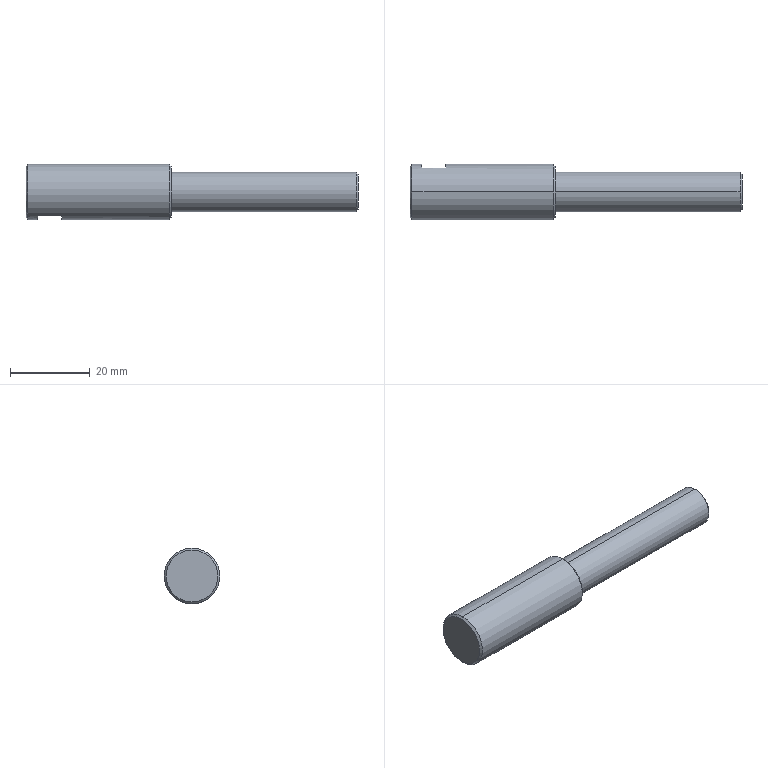Part | STEP file | 0243_216_Shaft | 1 solid | 19 faces | box 83.5 x 14 x 14 mm | volume 9237 mm3 | plane 9 | cone 6 | cylinder 4 | commonest cylinder face diameters 10 x2 14 x2
STEP:
#1=CARTESIAN_POINT('',(0.,0.,0.));
#2=DIRECTION('',(0.,0.,1.));
#3=DIRECTION('',(1.,0.,0.));
#4=AXIS2_PLACEMENT_3D('',#1,#2,#3);
#5=CARTESIAN_POINT('',(47.,0.,-4.5));
#6=VERTEX_POINT('',#5);
#7=CARTESIAN_POINT('',(47.,0.,4.5));
#8=VERTEX_POINT('',#7);
#9=CARTESIAN_POINT('',(47.,0.,0.));
#10=DIRECTION('',(1.,0.,0.));
#11=DIRECTION('',(0.,0.,1.));
#12=AXIS2_PLACEMENT_3D('',#9,#10,#11);
#13=CIRCLE('',#12,4.5);
#14=CARTESIAN_POINT('',(46.5,0.,0.));
#15=DIRECTION('',(-1.,0.,0.));
#16=DIRECTION('',(0.,0.,1.));
#17=AXIS2_PLACEMENT_3D('',#14,#15,#16);
#18=CONICAL_SURFACE('',#17,5.,0.7854);
#19=CARTESIAN_POINT('',(6.283,-0.5));
#20=DIRECTION('',(-1.,0.));
#21=VECTOR('',#20,1.);
#22=LINE('',#19,#21);
#23=(GEOMETRIC_REPRESENTATION_CONTEXT(2)PARAMETRIC_REPRESENTATION_CONTEXT()REPRESENTATION_CONTEXT('',''));
#24=DEFINITIONAL_REPRESENTATION('',(#22),#23);
#25=PCURVE('',#18,#24);
#26=CARTESIAN_POINT('',(47.,0.,0.));
#27=DIRECTION('',(-1.,0.,0.));
#28=DIRECTION('',(0.,0.,1.));
#29=AXIS2_PLACEMENT_3D('',#26,#27,#28);
#30=PLANE('',#29);
#31=CARTESIAN_POINT('',(4.5,0.));
#32=CARTESIAN_POINT('',(4.5,-7.794));
#33=CARTESIAN_POINT('',(-2.25,-3.897));
#34=CARTESIAN_POINT('',(-9.,0.));
#35=CARTESIAN_POINT('',(-2.25,3.897));
#36=CARTESIAN_POINT('',(4.5,7.794));
#37=CARTESIAN_POINT('',(4.5,0.));
#38=(BOUNDED_CURVE()B_SPLINE_CURVE(2,(#31,#32,#33,#34,#35,#36,#37),.UNSPECIFIED.,.T.,.F.)B_SPLINE_CURVE_WITH_KNOTS((1,2,2,2,2,1),(-2.094,0.,2.094,4.189,6.283,8.378),.UNSPECIFIED.)CURVE()GEOMETRIC_REPRESENTATION_ITEM()RATIONAL_B_SPLINE_CURVE((1.,0.5,1.,0.5,1.,0.5,1.))REPRESENTATION_ITEM(''));
#39=(GEOMETRIC_REPRESENTATION_CONTEXT(2)PARAMETRIC_REPRESENTATION_CONTEXT()REPRESENTATION_CONTEXT('',''));
#40=DEFINITIONAL_REPRESENTATION('',(#38),#39);
#41=PCURVE('',#30,#40);
#42=SURFACE_CURVE('',#13,(#25,#41),.PCURVE_S1.);
#43=EDGE_CURVE('',#6,#8,#42,.T.);
#44=ORIENTED_EDGE('',*,*,#43,.F.);
#45=CARTESIAN_POINT('',(46.5,0.,-5.));
#46=VERTEX_POINT('',#45);
#47=CARTESIAN_POINT('',(46.5,0.,-5.));
#48=DIRECTION('',(-0.7071,0.,-0.7071));
#49=VECTOR('',#48,1.);
#50=LINE('',#47,#49);
#51=CARTESIAN_POINT('',(3.142,0.));
#52=DIRECTION('',(0.,1.));
#53=VECTOR('',#52,1.);
#54=LINE('',#51,#53);
#55=(GEOMETRIC_REPRESENTATION_CONTEXT(2)PARAMETRIC_REPRESENTATION_CONTEXT()REPRESENTATION_CONTEXT('',''));
#56=DEFINITIONAL_REPRESENTATION('',(#54),#55);
#57=PCURVE('',#18,#56);
#58=CARTESIAN_POINT('',(46.5,0.,0.));
#59=DIRECTION('',(-1.,0.,0.));
#60=DIRECTION('',(0.,0.,1.));
#61=AXIS2_PLACEMENT_3D('',#58,#59,#60);
#62=CONICAL_SURFACE('',#61,5.,0.7854);
#63=CARTESIAN_POINT('',(3.142,0.));
#64=DIRECTION('',(0.,1.));
#65=VECTOR('',#64,1.);
#66=LINE('',#63,#65);
#67=(GEOMETRIC_REPRESENTATION_CONTEXT(2)PARAMETRIC_REPRESENTATION_CONTEXT()REPRESENTATION_CONTEXT('',''));
#68=DEFINITIONAL_REPRESENTATION('',(#66),#67);
#69=PCURVE('',#62,#68);
#70=SURFACE_CURVE('',#50,(#57,#69),.PCURVE_S1.);
#71=EDGE_CURVE('',#6,#46,#70,.T.);
#72=ORIENTED_EDGE('',*,*,#71,.T.);
#73=CARTESIAN_POINT('',(46.5,0.,5.));
#74=VERTEX_POINT('',#73);
#75=CARTESIAN_POINT('',(46.5,0.,0.));
#76=DIRECTION('',(-1.,0.,0.));
#77=DIRECTION('',(0.,0.,1.));
#78=AXIS2_PLACEMENT_3D('',#75,#76,#77);
#79=CIRCLE('',#78,5.);
#80=CARTESIAN_POINT('',(0.,0.));
#81=DIRECTION('',(1.,0.));
#82=VECTOR('',#81,1.);
#83=LINE('',#80,#82);
#84=(GEOMETRIC_REPRESENTATION_CONTEXT(2)PARAMETRIC_REPRESENTATION_CONTEXT()REPRESENTATION_CONTEXT('',''));
#85=DEFINITIONAL_REPRESENTATION('',(#83),#84);
#86=PCURVE('',#18,#85);
#87=CARTESIAN_POINT('',(-41.827,0.,0.));
#88=DIRECTION('',(-1.,0.,0.));
#89=DIRECTION('',(0.,0.,1.));
#90=AXIS2_PLACEMENT_3D('',#87,#88,#89);
#91=CYLINDRICAL_SURFACE('',#90,5.);
#92=CARTESIAN_POINT('',(0.,-88.327));
#93=DIRECTION('',(1.,0.));
#94=VECTOR('',#93,1.);
#95=LINE('',#92,#94);
#96=(GEOMETRIC_REPRESENTATION_CONTEXT(2)PARAMETRIC_REPRESENTATION_CONTEXT()REPRESENTATION_CONTEXT('',''));
#97=DEFINITIONAL_REPRESENTATION('',(#95),#96);
#98=PCURVE('',#91,#97);
#99=SURFACE_CURVE('',#79,(#86,#98),.PCURVE_S1.);
#100=EDGE_CURVE('',#74,#46,#99,.T.);
#101=ORIENTED_EDGE('',*,*,#100,.F.);
#102=CARTESIAN_POINT('',(46.5,0.,5.));
#103=DIRECTION('',(-0.7071,0.,0.7071));
#104=VECTOR('',#103,1.);
#105=LINE('',#102,#104);
#106=CARTESIAN_POINT('',(0.,0.));
#107=DIRECTION('',(0.,1.));
#108=VECTOR('',#107,1.);
#109=LINE('',#106,#108);
#110=(GEOMETRIC_REPRESENTATION_CONTEXT(2)PARAMETRIC_REPRESENTATION_CONTEXT()REPRESENTATION_CONTEXT('',''));
#111=DEFINITIONAL_REPRESENTATION('',(#109),#110);
#112=PCURVE('',#18,#111);
#113=CARTESIAN_POINT('',(6.283,0.));
#114=DIRECTION('',(0.,1.));
#115=VECTOR('',#114,1.);
#116=LINE('',#113,#115);
#117=(GEOMETRIC_REPRESENTATION_CONTEXT(2)PARAMETRIC_REPRESENTATION_CONTEXT()REPRESENTATION_CONTEXT('',''));
#118=DEFINITIONAL_REPRESENTATION('',(#116),#117);
#119=PCURVE('',#62,#118);
#120=SURFACE_CURVE('',#105,(#112,#119),.PCURVE_S1.);
#121=EDGE_CURVE('',#8,#74,#120,.T.);
#122=ORIENTED_EDGE('',*,*,#121,.F.);
#123=EDGE_LOOP('',(#44,#72,#101,#122));
#124=FACE_BOUND('',#123,.T.);
#125=ADVANCED_FACE('',(#124),#18,.T.);
#126=CARTESIAN_POINT('',(0.,0.,-6.5));
#127=VERTEX_POINT('',#126);
#128=CARTESIAN_POINT('',(0.,0.,6.5));
#129=VERTEX_POINT('',#128);
#130=CARTESIAN_POINT('',(0.,0.,0.));
#131=DIRECTION('',(1.,0.,0.));
#132=DIRECTION('',(0.,0.,1.));
#133=AXIS2_PLACEMENT_3D('',#130,#131,#132);
#134=CIRCLE('',#133,6.5);
#135=CARTESIAN_POINT('',(-0.5,0.,0.));
#136=DIRECTION('',(-1.,0.,0.));
#137=DIRECTION('',(0.,0.,1.));
#138=AXIS2_PLACEMENT_3D('',#135,#136,#137);
#139=CONICAL_SURFACE('',#138,7.,0.7854);
#140=CARTESIAN_POINT('',(6.283,-0.5));
#141=DIRECTION('',(-1.,0.));
#142=VECTOR('',#141,1.);
#143=LINE('',#140,#142);
#144=(GEOMETRIC_REPRESENTATION_CONTEXT(2)PARAMETRIC_REPRESENTATION_CONTEXT()REPRESENTATION_CONTEXT('',''));
#145=DEFINITIONAL_REPRESENTATION('',(#143),#144);
#146=PCURVE('',#139,#145);
#147=CARTESIAN_POINT('',(0.,5.,0.));
#148=DIRECTION('',(-1.,0.,0.));
#149=DIRECTION('',(0.,0.,1.));
#150=AXIS2_PLACEMENT_3D('',#147,#148,#149);
#151=PLANE('',#150);
#152=CARTESIAN_POINT('',(6.5,-5.));
#153=CARTESIAN_POINT('',(6.5,-16.258));
#154=CARTESIAN_POINT('',(-3.25,-10.629));
#155=CARTESIAN_POINT('',(-13.,-5.));
#156=CARTESIAN_POINT('',(-3.25,0.6292));
#157=CARTESIAN_POINT('',(6.5,6.258));
#158=CARTESIAN_POINT('',(6.5,-5.));
#159=(BOUNDED_CURVE()B_SPLINE_CURVE(2,(#152,#153,#154,#155,#156,#157,#158),.UNSPECIFIED.,.T.,.F.)B_SPLINE_CURVE_WITH_KNOTS((1,2,2,2,2,1),(-2.094,0.,2.094,4.189,6.283,8.378),.UNSPECIFIED.)CURVE()GEOMETRIC_REPRESENTATION_ITEM()RATIONAL_B_SPLINE_CURVE((1.,0.5,1.,0.5,1.,0.5,1.))REPRESENTATION_ITEM(''));
#160=(GEOMETRIC_REPRESENTATION_CONTEXT(2)PARAMETRIC_REPRESENTATION_CONTEXT()REPRESENTATION_CONTEXT('',''));
#161=DEFINITIONAL_REPRESENTATION('',(#159),#160);
#162=PCURVE('',#151,#161);
#163=SURFACE_CURVE('',#134,(#146,#162),.PCURVE_S1.);
#164=EDGE_CURVE('',#127,#129,#163,.T.);
#165=ORIENTED_EDGE('',*,*,#164,.F.);
#166=CARTESIAN_POINT('',(-0.5,0.,-7.));
#167=VERTEX_POINT('',#166);
#168=CARTESIAN_POINT('',(-0.5,0.,-7.));
#169=DIRECTION('',(-0.7071,0.,-0.7071));
#170=VECTOR('',#169,1.);
#171=LINE('',#168,#170);
#172=CARTESIAN_POINT('',(3.142,0.));
#173=DIRECTION('',(0.,1.));
#174=VECTOR('',#173,1.);
#175=LINE('',#172,#174);
#176=(GEOMETRIC_REPRESENTATION_CONTEXT(2)PARAMETRIC_REPRESENTATION_CONTEXT()REPRESENTATION_CONTEXT('',''));
#177=DEFINITIONAL_REPRESENTATION('',(#175),#176);
#178=PCURVE('',#139,#177);
#179=CARTESIAN_POINT('',(-0.5,0.,0.));
#180=DIRECTION('',(-1.,0.,0.));
#181=DIRECTION('',(0.,0.,1.));
#182=AXIS2_PLACEMENT_3D('',#179,#180,#181);
#183=CONICAL_SURFACE('',#182,7.,0.7854);
#184=CARTESIAN_POINT('',(3.142,0.));
#185=DIRECTION('',(0.,1.));
#186=VECTOR('',#185,1.);
#187=LINE('',#184,#186);
#188=(GEOMETRIC_REPRESENTATION_CONTEXT(2)PARAMETRIC_REPRESENTATION_CONTEXT()REPRESENTATION_CONTEXT('',''));
#189=DEFINITIONAL_REPRESENTATION('',(#187),#188);
#190=PCURVE('',#183,#189);
#191=SURFACE_CURVE('',#171,(#178,#190),.PCURVE_S1.);
#192=EDGE_CURVE('',#127,#167,#191,.T.);
#193=ORIENTED_EDGE('',*,*,#192,.T.);
#194=CARTESIAN_POINT('',(-0.5,0.,7.));
#195=VERTEX_POINT('',#194);
#196=CARTESIAN_POINT('',(-0.5,0.,0.));
#197=DIRECTION('',(-1.,0.,0.));
#198=DIRECTION('',(0.,0.,1.));
#199=AXIS2_PLACEMENT_3D('',#196,#197,#198);
#200=CIRCLE('',#199,7.);
#201=CARTESIAN_POINT('',(0.,0.));
#202=DIRECTION('',(1.,0.));
#203=VECTOR('',#202,1.);
#204=LINE('',#201,#203);
#205=(GEOMETRIC_REPRESENTATION_CONTEXT(2)PARAMETRIC_REPRESENTATION_CONTEXT()REPRESENTATION_CONTEXT('',''));
#206=DEFINITIONAL_REPRESENTATION('',(#204),#205);
#207=PCURVE('',#139,#206);
#208=CARTESIAN_POINT('',(-41.827,0.,0.));
#209=DIRECTION('',(-1.,0.,0.));
#210=DIRECTION('',(0.,0.,1.));
#211=AXIS2_PLACEMENT_3D('',#208,#209,#210);
#212=CYLINDRICAL_SURFACE('',#211,7.);
#213=CARTESIAN_POINT('',(0.,-41.327));
#214=DIRECTION('',(1.,0.));
#215=VECTOR('',#214,1.);
#216=LINE('',#213,#215);
#217=(GEOMETRIC_REPRESENTATION_CONTEXT(2)PARAMETRIC_REPRESENTATION_CONTEXT()REPRESENTATION_CONTEXT('',''));
#218=DEFINITIONAL_REPRESENTATION('',(#216),#217);
#219=PCURVE('',#212,#218);
#220=SURFACE_CURVE('',#200,(#207,#219),.PCURVE_S1.);
#221=EDGE_CURVE('',#195,#167,#220,.T.);
#222=ORIENTED_EDGE('',*,*,#221,.F.);
#223=CARTESIAN_POINT('',(-0.5,0.,7.));
#224=DIRECTION('',(-0.7071,0.,0.7071));
#225=VECTOR('',#224,1.);
#226=LINE('',#223,#225);
#227=CARTESIAN_POINT('',(0.,0.));
#228=DIRECTION('',(0.,1.));
#229=VECTOR('',#228,1.);
#230=LINE('',#227,#229);
#231=(GEOMETRIC_REPRESENTATION_CONTEXT(2)PARAMETRIC_REPRESENTATION_CONTEXT()REPRESENTATION_CONTEXT('',''));
#232=DEFINITIONAL_REPRESENTATION('',(#230),#231);
#233=PCURVE('',#139,#232);
#234=CARTESIAN_POINT('',(6.283,0.));
#235=DIRECTION('',(0.,1.));
#236=VECTOR('',#235,1.);
#237=LINE('',#234,#236);
#238=(GEOMETRIC_REPRESENTATION_CONTEXT(2)PARAMETRIC_REPRESENTATION_CONTEXT()REPRESENTATION_CONTEXT('',''));
#239=DEFINITIONAL_REPRESENTATION('',(#237),#238);
#240=PCURVE('',#183,#239);
#241=SURFACE_CURVE('',#226,(#233,#240),.PCURVE_S1.);
#242=EDGE_CURVE('',#129,#195,#241,.T.);
#243=ORIENTED_EDGE('',*,*,#242,.F.);
#244=EDGE_LOOP('',(#165,#193,#222,#243));
#245=FACE_BOUND('',#244,.T.);
#246=ADVANCED_FACE('',(#245),#139,.T.);
#247=CARTESIAN_POINT('',(-36.5,0.,6.5));
#248=VERTEX_POINT('',#247);
#249=CARTESIAN_POINT('',(-36.5,0.,-6.5));
#250=VERTEX_POINT('',#249);
#251=CARTESIAN_POINT('',(-36.5,0.,0.));
#252=DIRECTION('',(-1.,0.,0.));
#253=DIRECTION('',(0.,0.,-1.));
#254=AXIS2_PLACEMENT_3D('',#251,#252,#253);
#255=CIRCLE('',#254,6.5);
#256=CARTESIAN_POINT('',(-36.5,0.,0.));
#257=DIRECTION('',(1.,0.,0.));
#258=DIRECTION('',(0.,0.,-1.));
#259=AXIS2_PLACEMENT_3D('',#256,#257,#258);
#260=CONICAL_SURFACE('',#259,6.5,0.7854);
#261=CARTESIAN_POINT('',(6.283,0.));
#262=DIRECTION('',(-1.,0.));
#263=VECTOR('',#262,1.);
#264=LINE('',#261,#263);
#265=(GEOMETRIC_REPRESENTATION_CONTEXT(2)PARAMETRIC_REPRESENTATION_CONTEXT()REPRESENTATION_CONTEXT('',''));
#266=DEFINITIONAL_REPRESENTATION('',(#264),#265);
#267=PCURVE('',#260,#266);
#268=CARTESIAN_POINT('',(-36.5,7.,0.));
#269=DIRECTION('',(1.,0.,0.));
#270=DIRECTION('',(0.,0.,-1.));
#271=AXIS2_PLACEMENT_3D('',#268,#269,#270);
#272=PLANE('',#271);
#273=CARTESIAN_POINT('',(6.5,-7.));
#274=CARTESIAN_POINT('',(6.5,-18.258));
#275=CARTESIAN_POINT('',(-3.25,-12.629));
#276=CARTESIAN_POINT('',(-13.,-7.));
#277=CARTESIAN_POINT('',(-3.25,-1.371));
#278=CARTESIAN_POINT('',(6.5,4.258));
#279=CARTESIAN_POINT('',(6.5,-7.));
#280=(BOUNDED_CURVE()B_SPLINE_CURVE(2,(#273,#274,#275,#276,#277,#278,#279),.UNSPECIFIED.,.T.,.F.)B_SPLINE_CURVE_WITH_KNOTS((1,2,2,2,2,1),(-2.094,0.,2.094,4.189,6.283,8.378),.UNSPECIFIED.)CURVE()GEOMETRIC_REPRESENTATION_ITEM()RATIONAL_B_SPLINE_CURVE((1.,0.5,1.,0.5,1.,0.5,1.))REPRESENTATION_ITEM(''));
#281=(GEOMETRIC_REPRESENTATION_CONTEXT(2)PARAMETRIC_REPRESENTATION_CONTEXT()REPRESENTATION_CONTEXT('',''));
#282=DEFINITIONAL_REPRESENTATION('',(#280),#281);
#283=PCURVE('',#272,#282);
#284=SURFACE_CURVE('',#255,(#267,#283),.PCURVE_S1.);
#285=EDGE_CURVE('',#248,#250,#284,.T.);
#286=ORIENTED_EDGE('',*,*,#285,.F.);
#287=CARTESIAN_POINT('',(-36.,0.,7.));
#288=VERTEX_POINT('',#287);
#289=CARTESIAN_POINT('',(-36.5,0.,6.5));
#290=DIRECTION('',(0.7071,0.,0.7071));
#291=VECTOR('',#290,1.);
#292=LINE('',#289,#291);
#293=CARTESIAN_POINT('',(3.142,0.));
#294=DIRECTION('',(0.,1.));
#295=VECTOR('',#294,1.);
#296=LINE('',#293,#295);
#297=(GEOMETRIC_REPRESENTATION_CONTEXT(2)PARAMETRIC_REPRESENTATION_CONTEXT()REPRESENTATION_CONTEXT('',''));
#298=DEFINITIONAL_REPRESENTATION('',(#296),#297);
#299=PCURVE('',#260,#298);
#300=CARTESIAN_POINT('',(-36.5,0.,0.));
#301=DIRECTION('',(1.,0.,0.));
#302=DIRECTION('',(0.,0.,-1.));
#303=AXIS2_PLACEMENT_3D('',#300,#301,#302);
#304=CONICAL_SURFACE('',#303,6.5,0.7854);
#305=CARTESIAN_POINT('',(3.142,0.));
#306=DIRECTION('',(0.,1.));
#307=VECTOR('',#306,1.);
#308=LINE('',#305,#307);
#309=(GEOMETRIC_REPRESENTATION_CONTEXT(2)PARAMETRIC_REPRESENTATION_CONTEXT()REPRESENTATION_CONTEXT('',''));
#310=DEFINITIONAL_REPRESENTATION('',(#308),#309);
#311=PCURVE('',#304,#310);
#312=SURFACE_CURVE('',#292,(#299,#311),.PCURVE_S1.);
#313=EDGE_CURVE('',#248,#288,#312,.T.);
#314=ORIENTED_EDGE('',*,*,#313,.T.);
#315=CARTESIAN_POINT('',(-36.,0.,-7.));
#316=VERTEX_POINT('',#315);
#317=CARTESIAN_POINT('',(-36.,0.,0.));
#318=DIRECTION('',(1.,0.,0.));
#319=DIRECTION('',(0.,0.,-1.));
#320=AXIS2_PLACEMENT_3D('',#317,#318,#319);
#321=CIRCLE('',#320,7.);
#322=CARTESIAN_POINT('',(0.,0.5));
#323=DIRECTION('',(1.,0.));
#324=VECTOR('',#323,1.);
#325=LINE('',#322,#324);
#326=(GEOMETRIC_REPRESENTATION_CONTEXT(2)PARAMETRIC_REPRESENTATION_CONTEXT()REPRESENTATION_CONTEXT('',''));
#327=DEFINITIONAL_REPRESENTATION('',(#325),#326);
#328=PCURVE('',#260,#327);
#329=CARTESIAN_POINT('',(3.142,-5.827));
#330=DIRECTION('',(-1.,0.));
#331=VECTOR('',#330,1.);
#332=LINE('',#329,#331);
#333=(GEOMETRIC_REPRESENTATION_CONTEXT(2)PARAMETRIC_REPRESENTATION_CONTEXT()REPRESENTATION_CONTEXT('',''));
#334=DEFINITIONAL_REPRESENTATION('',(#332),#333);
#335=PCURVE('',#212,#334);
#336=SURFACE_CURVE('',#321,(#328,#335),.PCURVE_S1.);
#337=EDGE_CURVE('',#316,#288,#336,.T.);
#338=ORIENTED_EDGE('',*,*,#337,.F.);
#339=CARTESIAN_POINT('',(-36.5,0.,-6.5));
#340=DIRECTION('',(0.7071,0.,-0.7071));
#341=VECTOR('',#340,1.);
#342=LINE('',#339,#341);
#343=CARTESIAN_POINT('',(0.,0.));
#344=DIRECTION('',(0.,1.));
#345=VECTOR('',#344,1.);
#346=LINE('',#343,#345);
#347=(GEOMETRIC_REPRESENTATION_CONTEXT(2)PARAMETRIC_REPRESENTATION_CONTEXT()REPRESENTATION_CONTEXT('',''));
#348=DEFINITIONAL_REPRESENTATION('',(#346),#347);
#349=PCURVE('',#260,#348);
#350=CARTESIAN_POINT('',(6.283,0.));
#351=DIRECTION('',(0.,1.));
#352=VECTOR('',#351,1.);
#353=LINE('',#350,#352);
#354=(GEOMETRIC_REPRESENTATION_CONTEXT(2)PARAMETRIC_REPRESENTATION_CONTEXT()REPRESENTATION_CONTEXT('',''));
#355=DEFINITIONAL_REPRESENTATION('',(#353),#354);
#356=PCURVE('',#304,#355);
#357=SURFACE_CURVE('',#342,(#349,#356),.PCURVE_S1.);
#358=EDGE_CURVE('',#250,#316,#357,.T.);
#359=ORIENTED_EDGE('',*,*,#358,.F.);
#360=EDGE_LOOP('',(#286,#314,#338,#359));
#361=FACE_BOUND('',#360,.T.);
#362=ADVANCED_FACE('',(#361),#260,.T.);
#363=CARTESIAN_POINT('',(-27.5,6.,-3.606));
#364=VERTEX_POINT('',#363);
#365=CARTESIAN_POINT('',(-27.5,6.,3.606));
#366=VERTEX_POINT('',#365);
#367=CARTESIAN_POINT('',(-27.5,0.,0.));
#368=DIRECTION('',(1.,0.,0.));
#369=DIRECTION('',(0.,0.,-1.));
#370=AXIS2_PLACEMENT_3D('',#367,#368,#369);
#371=CIRCLE('',#370,7.);
#372=CARTESIAN_POINT('',(3.142,-14.327));
#373=DIRECTION('',(-1.,0.));
#374=VECTOR('',#373,1.);
#375=LINE('',#372,#374);
#376=(GEOMETRIC_REPRESENTATION_CONTEXT(2)PARAMETRIC_REPRESENTATION_CONTEXT()REPRESENTATION_CONTEXT('',''));
#377=DEFINITIONAL_REPRESENTATION('',(#375),#376);
#378=PCURVE('',#212,#377);
#379=CARTESIAN_POINT('',(-27.5,7.,-7.));
#380=DIRECTION('',(1.,0.,0.));
#381=DIRECTION('',(0.,0.,-1.));
#382=AXIS2_PLACEMENT_3D('',#379,#380,#381);
#383=PLANE('',#382);
#384=CARTESIAN_POINT('',(-7.,-7.));
#385=DIRECTION('',(1.,0.));
#386=AXIS2_PLACEMENT_2D('',#384,#385);
#387=CIRCLE('',#386,7.);
#388=(GEOMETRIC_REPRESENTATION_CONTEXT(2)PARAMETRIC_REPRESENTATION_CONTEXT()REPRESENTATION_CONTEXT('',''));
#389=DEFINITIONAL_REPRESENTATION('',(#387),#388);
#390=PCURVE('',#383,#389);
#391=SURFACE_CURVE('',#371,(#378,#390),.PCURVE_S1.);
#392=EDGE_CURVE('',#364,#366,#391,.T.);
#393=ORIENTED_EDGE('',*,*,#392,.T.);
#394=CARTESIAN_POINT('',(-33.5,6.,3.606));
#395=VERTEX_POINT('',#394);
#396=CARTESIAN_POINT('',(-41.827,6.,3.606));
#397=DIRECTION('',(-1.,0.,0.));
#398=VECTOR('',#397,1.);
#399=LINE('',#396,#398);
#400=CARTESIAN_POINT('',(1.03,0.));
#401=DIRECTION('',(0.,1.));
#402=VECTOR('',#401,1.);
#403=LINE('',#400,#402);
#404=(GEOMETRIC_REPRESENTATION_CONTEXT(2)PARAMETRIC_REPRESENTATION_CONTEXT()REPRESENTATION_CONTEXT('',''));
#405=DEFINITIONAL_REPRESENTATION('',(#403),#404);
#406=PCURVE('',#212,#405);
#407=CARTESIAN_POINT('',(-33.5,6.,-7.));
#408=DIRECTION('',(0.,-1.,0.));
#409=DIRECTION('',(1.,0.,0.));
#410=AXIS2_PLACEMENT_3D('',#407,#408,#409);
#411=PLANE('',#410);
#412=CARTESIAN_POINT('',(-8.327,10.606));
#413=DIRECTION('',(-1.,0.));
#414=VECTOR('',#413,1.);
#415=LINE('',#412,#414);
#416=(GEOMETRIC_REPRESENTATION_CONTEXT(2)PARAMETRIC_REPRESENTATION_CONTEXT()REPRESENTATION_CONTEXT('',''));
#417=DEFINITIONAL_REPRESENTATION('',(#415),#416);
#418=PCURVE('',#411,#417);
#419=SURFACE_CURVE('',#399,(#406,#418),.PCURVE_S1.);
#420=EDGE_CURVE('',#366,#395,#419,.T.);
#421=ORIENTED_EDGE('',*,*,#420,.T.);
#422=CARTESIAN_POINT('',(-33.5,6.,-3.606));
#423=VERTEX_POINT('',#422);
#424=CARTESIAN_POINT('',(-33.5,0.,0.));
#425=DIRECTION('',(-1.,0.,0.));
#426=DIRECTION('',(0.,0.,1.));
#427=AXIS2_PLACEMENT_3D('',#424,#425,#426);
#428=CIRCLE('',#427,7.);
#429=CARTESIAN_POINT('',(0.,-8.327));
#430=DIRECTION('',(1.,0.));
#431=VECTOR('',#430,1.);
#432=LINE('',#429,#431);
#433=(GEOMETRIC_REPRESENTATION_CONTEXT(2)PARAMETRIC_REPRESENTATION_CONTEXT()REPRESENTATION_CONTEXT('',''));
#434=DEFINITIONAL_REPRESENTATION('',(#432),#433);
#435=PCURVE('',#212,#434);
#436=CARTESIAN_POINT('',(-33.5,7.,-7.));
#437=DIRECTION('',(-1.,0.,0.));
#438=DIRECTION('',(0.,0.,1.));
#439=AXIS2_PLACEMENT_3D('',#436,#437,#438);
#440=PLANE('',#439);
#441=CARTESIAN_POINT('',(7.,-7.));
#442=DIRECTION('',(1.,0.));
#443=AXIS2_PLACEMENT_2D('',#441,#442);
#444=CIRCLE('',#443,7.);
#445=(GEOMETRIC_REPRESENTATION_CONTEXT(2)PARAMETRIC_REPRESENTATION_CONTEXT()REPRESENTATION_CONTEXT('',''));
#446=DEFINITIONAL_REPRESENTATION('',(#444),#445);
#447=PCURVE('',#440,#446);
#448=SURFACE_CURVE('',#428,(#435,#447),.PCURVE_S1.);
#449=EDGE_CURVE('',#395,#423,#448,.T.);
#450=ORIENTED_EDGE('',*,*,#449,.T.);
#451=CARTESIAN_POINT('',(-41.827,6.,-3.606));
#452=DIRECTION('',(1.,0.,0.));
#453=VECTOR('',#452,1.);
#454=LINE('',#451,#453);
#455=CARTESIAN_POINT('',(2.112,0.));
#456=DIRECTION('',(0.,-1.));
#457=VECTOR('',#456,1.);
#458=LINE('',#455,#457);
#459=(GEOMETRIC_REPRESENTATION_CONTEXT(2)PARAMETRIC_REPRESENTATION_CONTEXT()REPRESENTATION_CONTEXT('',''));
#460=DEFINITIONAL_REPRESENTATION('',(#458),#459);
#461=PCURVE('',#212,#460);
#462=CARTESIAN_POINT('',(-8.327,3.394));
#463=DIRECTION('',(1.,0.));
#464=VECTOR('',#463,1.);
#465=LINE('',#462,#464);
#466=(GEOMETRIC_REPRESENTATION_CONTEXT(2)PARAMETRIC_REPRESENTATION_CONTEXT()REPRESENTATION_CONTEXT('',''));
#467=DEFINITIONAL_REPRESENTATION('',(#465),#466);
#468=PCURVE('',#411,#467);
#469=SURFACE_CURVE('',#454,(#461,#468),.PCURVE_S1.);
#470=EDGE_CURVE('',#423,#364,#469,.T.);
#471=ORIENTED_EDGE('',*,*,#470,.T.);
#472=EDGE_LOOP('',(#393,#421,#450,#471));
#473=FACE_BOUND('',#472,.T.);
#474=ORIENTED_EDGE('',*,*,#221,.T.);
#475=CARTESIAN_POINT('',(-27.5,0.,-7.));
#476=VERTEX_POINT('',#475);
#477=CARTESIAN_POINT('',(-41.827,0.,-7.));
#478=DIRECTION('',(-1.,0.,0.));
#479=VECTOR('',#478,1.);
#480=LINE('',#477,#479);
#481=CARTESIAN_POINT('',(3.142,0.));
#482=DIRECTION('',(0.,1.));
#483=VECTOR('',#482,1.);
#484=LINE('',#481,#483);
#485=(GEOMETRIC_REPRESENTATION_CONTEXT(2)PARAMETRIC_REPRESENTATION_CONTEXT()REPRESENTATION_CONTEXT('',''));
#486=DEFINITIONAL_REPRESENTATION('',(#484),#485);
#487=PCURVE('',#212,#486);
#488=CARTESIAN_POINT('',(-41.827,0.,0.));
#489=DIRECTION('',(-1.,0.,0.));
#490=DIRECTION('',(0.,0.,1.));
#491=AXIS2_PLACEMENT_3D('',#488,#489,#490);
#492=CYLINDRICAL_SURFACE('',#491,7.);
#493=CARTESIAN_POINT('',(3.142,0.));
#494=DIRECTION('',(0.,1.));
#495=VECTOR('',#494,1.);
#496=LINE('',#493,#495);
#497=(GEOMETRIC_REPRESENTATION_CONTEXT(2)PARAMETRIC_REPRESENTATION_CONTEXT()REPRESENTATION_CONTEXT('',''));
#498=DEFINITIONAL_REPRESENTATION('',(#496),#497);
#499=PCURVE('',#492,#498);
#500=SURFACE_CURVE('',#480,(#487,#499),.PCURVE_S1.);
#501=EDGE_CURVE('',#167,#476,#500,.T.);
#502=ORIENTED_EDGE('',*,*,#501,.T.);
#503=CARTESIAN_POINT('',(-27.5,3.606,-6.));
#504=VERTEX_POINT('',#503);
#505=CARTESIAN_POINT('',(-27.5,0.,0.));
#506=DIRECTION('',(1.,0.,0.));
#507=DIRECTION('',(0.,0.,-1.));
#508=AXIS2_PLACEMENT_3D('',#505,#506,#507);
#509=CIRCLE('',#508,7.);
#510=CARTESIAN_POINT('',(3.142,-14.327));
#511=DIRECTION('',(-1.,0.));
#512=VECTOR('',#511,1.);
#513=LINE('',#510,#512);
#514=(GEOMETRIC_REPRESENTATION_CONTEXT(2)PARAMETRIC_REPRESENTATION_CONTEXT()REPRESENTATION_CONTEXT('',''));
#515=DEFINITIONAL_REPRESENTATION('',(#513),#514);
#516=PCURVE('',#212,#515);
#517=CARTESIAN_POINT('',(-27.5,-7.,-7.));
#518=DIRECTION('',(1.,0.,0.));
#519=DIRECTION('',(0.,0.,-1.));
#520=AXIS2_PLACEMENT_3D('',#517,#518,#519);
#521=PLANE('',#520);
#522=CARTESIAN_POINT('',(-7.,7.));
#523=DIRECTION('',(1.,0.));
#524=AXIS2_PLACEMENT_2D('',#522,#523);
#525=CIRCLE('',#524,7.);
#526=(GEOMETRIC_REPRESENTATION_CONTEXT(2)PARAMETRIC_REPRESENTATION_CONTEXT()REPRESENTATION_CONTEXT('',''));
#527=DEFINITIONAL_REPRESENTATION('',(#525),#526);
#528=PCURVE('',#521,#527);
#529=SURFACE_CURVE('',#509,(#516,#528),.PCURVE_S1.);
#530=EDGE_CURVE('',#476,#504,#529,.T.);
#531=ORIENTED_EDGE('',*,*,#530,.T.);
#532=CARTESIAN_POINT('',(-33.5,3.606,-6.));
#533=VERTEX_POINT('',#532);
#534=CARTESIAN_POINT('',(-41.827,3.606,-6.));
#535=DIRECTION('',(-1.,0.,0.));
#536=VECTOR('',#535,1.);
#537=LINE('',#534,#536);
#538=CARTESIAN_POINT('',(2.6,0.));
#539=DIRECTION('',(0.,1.));
#540=VECTOR('',#539,1.);
#541=LINE('',#538,#540);
#542=(GEOMETRIC_REPRESENTATION_CONTEXT(2)PARAMETRIC_REPRESENTATION_CONTEXT()REPRESENTATION_CONTEXT('',''));
#543=DEFINITIONAL_REPRESENTATION('',(#541),#542);
#544=PCURVE('',#212,#543);
#545=CARTESIAN_POINT('',(-33.5,-7.,-6.));
#546=DIRECTION('',(0.,0.,1.));
#547=DIRECTION('',(0.,-1.,0.));
#548=AXIS2_PLACEMENT_3D('',#545,#546,#547);
#549=PLANE('',#548);
#550=CARTESIAN_POINT('',(-10.606,-8.327));
#551=DIRECTION('',(0.,-1.));
#552=VECTOR('',#551,1.);
#553=LINE('',#550,#552);
#554=(GEOMETRIC_REPRESENTATION_CONTEXT(2)PARAMETRIC_REPRESENTATION_CONTEXT()REPRESENTATION_CONTEXT('',''));
#555=DEFINITIONAL_REPRESENTATION('',(#553),#554);
#556=PCURVE('',#549,#555);
#557=SURFACE_CURVE('',#537,(#544,#556),.PCURVE_S1.);
#558=EDGE_CURVE('',#504,#533,#557,.T.);
#559=ORIENTED_EDGE('',*,*,#558,.T.);
#560=CARTESIAN_POINT('',(-33.5,0.,-7.));
#561=VERTEX_POINT('',#560);
#562=CARTESIAN_POINT('',(-33.5,0.,0.));
#563=DIRECTION('',(-1.,0.,0.));
#564=DIRECTION('',(0.,0.,1.));
#565=AXIS2_PLACEMENT_3D('',#562,#563,#564);
#566=CIRCLE('',#565,7.);
#567=CARTESIAN_POINT('',(0.,-8.327));
#568=DIRECTION('',(1.,0.));
#569=VECTOR('',#568,1.);
#570=LINE('',#567,#569);
#571=(GEOMETRIC_REPRESENTATION_CONTEXT(2)PARAMETRIC_REPRESENTATION_CONTEXT()REPRESENTATION_CONTEXT('',''));
#572=DEFINITIONAL_REPRESENTATION('',(#570),#571);
#573=PCURVE('',#212,#572);
#574=CARTESIAN_POINT('',(-33.5,-7.,-7.));
#575=DIRECTION('',(-1.,0.,0.));
#576=DIRECTION('',(0.,0.,1.));
#577=AXIS2_PLACEMENT_3D('',#574,#575,#576);
#578=PLANE('',#577);
#579=CARTESIAN_POINT('',(7.,7.));
#580=DIRECTION('',(1.,0.));
#581=AXIS2_PLACEMENT_2D('',#579,#580);
#582=CIRCLE('',#581,7.);
#583=(GEOMETRIC_REPRESENTATION_CONTEXT(2)PARAMETRIC_REPRESENTATION_CONTEXT()REPRESENTATION_CONTEXT('',''));
#584=DEFINITIONAL_REPRESENTATION('',(#582),#583);
#585=PCURVE('',#578,#584);
#586=SURFACE_CURVE('',#566,(#573,#585),.PCURVE_S1.);
#587=EDGE_CURVE('',#533,#561,#586,.T.);
#588=ORIENTED_EDGE('',*,*,#587,.T.);
#589=CARTESIAN_POINT('',(-41.827,0.,-7.));
#590=DIRECTION('',(-1.,0.,0.));
#591=VECTOR('',#590,1.);
#592=LINE('',#589,#591);
#593=CARTESIAN_POINT('',(3.142,0.));
#594=DIRECTION('',(0.,1.));
#595=VECTOR('',#594,1.);
#596=LINE('',#593,#595);
#597=(GEOMETRIC_REPRESENTATION_CONTEXT(2)PARAMETRIC_REPRESENTATION_CONTEXT()REPRESENTATION_CONTEXT('',''));
#598=DEFINITIONAL_REPRESENTATION('',(#596),#597);
#599=PCURVE('',#212,#598);
#600=CARTESIAN_POINT('',(3.142,0.));
#601=DIRECTION('',(0.,1.));
#602=VECTOR('',#601,1.);
#603=LINE('',#600,#602);
#604=(GEOMETRIC_REPRESENTATION_CONTEXT(2)PARAMETRIC_REPRESENTATION_CONTEXT()REPRESENTATION_CONTEXT('',''));
#605=DEFINITIONAL_REPRESENTATION('',(#603),#604);
#606=PCURVE('',#492,#605);
#607=SURFACE_CURVE('',#592,(#599,#606),.PCURVE_S1.);
#608=EDGE_CURVE('',#561,#316,#607,.T.);
#609=ORIENTED_EDGE('',*,*,#608,.T.);
#610=ORIENTED_EDGE('',*,*,#337,.T.);
#611=CARTESIAN_POINT('',(-41.827,0.,7.));
#612=DIRECTION('',(-1.,0.,0.));
#613=VECTOR('',#612,1.);
#614=LINE('',#611,#613);
#615=CARTESIAN_POINT('',(0.,0.));
#616=DIRECTION('',(0.,1.));
#617=VECTOR('',#616,1.);
#618=LINE('',#615,#617);
#619=(GEOMETRIC_REPRESENTATION_CONTEXT(2)PARAMETRIC_REPRESENTATION_CONTEXT()REPRESENTATION_CONTEXT('',''));
#620=DEFINITIONAL_REPRESENTATION('',(#618),#619);
#621=PCURVE('',#212,#620);
#622=CARTESIAN_POINT('',(6.283,0.));
#623=DIRECTION('',(0.,1.));
#624=VECTOR('',#623,1.);
#625=LINE('',#622,#624);
#626=(GEOMETRIC_REPRESENTATION_CONTEXT(2)PARAMETRIC_REPRESENTATION_CONTEXT()REPRESENTATION_CONTEXT('',''));
#627=DEFINITIONAL_REPRESENTATION('',(#625),#626);
#628=PCURVE('',#492,#627);
#629=SURFACE_CURVE('',#614,(#621,#628),.PCURVE_S1.);
#630=EDGE_CURVE('',#195,#288,#629,.T.);
#631=ORIENTED_EDGE('',*,*,#630,.F.);
#632=EDGE_LOOP('',(#474,#502,#531,#559,#588,#609,#610,#631));
#633=FACE_BOUND('',#632,.T.);
#634=ADVANCED_FACE('',(#473,#633),#212,.T.);
#635=ORIENTED_EDGE('',*,*,#100,.T.);
#636=CARTESIAN_POINT('',(0.,0.,-5.));
#637=VERTEX_POINT('',#636);
#638=CARTESIAN_POINT('',(-41.827,0.,-5.));
#639=DIRECTION('',(-1.,0.,0.));
#640=VECTOR('',#639,1.);
#641=LINE('',#638,#640);
#642=CARTESIAN_POINT('',(3.142,0.));
#643=DIRECTION('',(0.,1.));
#644=VECTOR('',#643,1.);
#645=LINE('',#642,#644);
#646=(GEOMETRIC_REPRESENTATION_CONTEXT(2)PARAMETRIC_REPRESENTATION_CONTEXT()REPRESENTATION_CONTEXT('',''));
#647=DEFINITIONAL_REPRESENTATION('',(#645),#646);
#648=PCURVE('',#91,#647);
#649=CARTESIAN_POINT('',(-41.827,0.,0.));
#650=DIRECTION('',(-1.,0.,0.));
#651=DIRECTION('',(0.,0.,1.));
#652=AXIS2_PLACEMENT_3D('',#649,#650,#651);
#653=CYLINDRICAL_SURFACE('',#652,5.);
#654=CARTESIAN_POINT('',(3.142,0.));
#655=DIRECTION('',(0.,1.));
#656=VECTOR('',#655,1.);
#657=LINE('',#654,#656);
#658=(GEOMETRIC_REPRESENTATION_CONTEXT(2)PARAMETRIC_REPRESENTATION_CONTEXT()REPRESENTATION_CONTEXT('',''));
#659=DEFINITIONAL_REPRESENTATION('',(#657),#658);
#660=PCURVE('',#653,#659);
#661=SURFACE_CURVE('',#641,(#648,#660),.PCURVE_S1.);
#662=EDGE_CURVE('',#46,#637,#661,.T.);
#663=ORIENTED_EDGE('',*,*,#662,.T.);
#664=CARTESIAN_POINT('',(0.,0.,5.));
#665=VERTEX_POINT('',#664);
#666=CARTESIAN_POINT('',(0.,0.,0.));
#667=DIRECTION('',(-1.,0.,0.));
#668=DIRECTION('',(0.,0.,1.));
#669=AXIS2_PLACEMENT_3D('',#666,#667,#668);
#670=CIRCLE('',#669,5.);
#671=CARTESIAN_POINT('',(0.,-41.827));
#672=DIRECTION('',(1.,0.));
#673=VECTOR('',#672,1.);
#674=LINE('',#671,#673);
#675=(GEOMETRIC_REPRESENTATION_CONTEXT(2)PARAMETRIC_REPRESENTATION_CONTEXT()REPRESENTATION_CONTEXT('',''));
#676=DEFINITIONAL_REPRESENTATION('',(#674),#675);
#677=PCURVE('',#91,#676);
#678=CARTESIAN_POINT('',(0.,-5.));
#679=DIRECTION('',(1.,0.));
#680=AXIS2_PLACEMENT_2D('',#678,#679);
#681=CIRCLE('',#680,5.);
#682=(GEOMETRIC_REPRESENTATION_CONTEXT(2)PARAMETRIC_REPRESENTATION_CONTEXT()REPRESENTATION_CONTEXT('',''));
#683=DEFINITIONAL_REPRESENTATION('',(#681),#682);
#684=PCURVE('',#151,#683);
#685=SURFACE_CURVE('',#670,(#677,#684),.PCURVE_S1.);
#686=EDGE_CURVE('',#665,#637,#685,.T.);
#687=ORIENTED_EDGE('',*,*,#686,.F.);
#688=CARTESIAN_POINT('',(-41.827,0.,5.));
#689=DIRECTION('',(-1.,0.,0.));
#690=VECTOR('',#689,1.);
#691=LINE('',#688,#690);
#692=CARTESIAN_POINT('',(0.,0.));
#693=DIRECTION('',(0.,1.));
#694=VECTOR('',#693,1.);
#695=LINE('',#692,#694);
#696=(GEOMETRIC_REPRESENTATION_CONTEXT(2)PARAMETRIC_REPRESENTATION_CONTEXT()REPRESENTATION_CONTEXT('',''));
#697=DEFINITIONAL_REPRESENTATION('',(#695),#696);
#698=PCURVE('',#91,#697);
#699=CARTESIAN_POINT('',(6.283,0.));
#700=DIRECTION('',(0.,1.));
#701=VECTOR('',#700,1.);
#702=LINE('',#699,#701);
#703=(GEOMETRIC_REPRESENTATION_CONTEXT(2)PARAMETRIC_REPRESENTATION_CONTEXT()REPRESENTATION_CONTEXT('',''));
#704=DEFINITIONAL_REPRESENTATION('',(#702),#703);
#705=PCURVE('',#653,#704);
#706=SURFACE_CURVE('',#691,(#698,#705),.PCURVE_S1.);
#707=EDGE_CURVE('',#74,#665,#706,.T.);
#708=ORIENTED_EDGE('',*,*,#707,.F.);
#709=EDGE_LOOP('',(#635,#663,#687,#708));
#710=FACE_BOUND('',#709,.T.);
#711=ADVANCED_FACE('',(#710),#91,.T.);
#712=CARTESIAN_POINT('',(47.,0.,0.));
#713=DIRECTION('',(1.,0.,0.));
#714=DIRECTION('',(0.,0.,1.));
#715=AXIS2_PLACEMENT_3D('',#712,#713,#714);
#716=CIRCLE('',#715,4.5);
#717=CARTESIAN_POINT('',(4.5,0.));
#718=CARTESIAN_POINT('',(4.5,-7.794));
#719=CARTESIAN_POINT('',(-2.25,-3.897));
#720=CARTESIAN_POINT('',(-9.,0.));
#721=CARTESIAN_POINT('',(-2.25,3.897));
#722=CARTESIAN_POINT('',(4.5,7.794));
#723=CARTESIAN_POINT('',(4.5,0.));
#724=(BOUNDED_CURVE()B_SPLINE_CURVE(2,(#717,#718,#719,#720,#721,#722,#723),.UNSPECIFIED.,.T.,.F.)B_SPLINE_CURVE_WITH_KNOTS((1,2,2,2,2,1),(-2.094,0.,2.094,4.189,6.283,8.378),.UNSPECIFIED.)CURVE()GEOMETRIC_REPRESENTATION_ITEM()RATIONAL_B_SPLINE_CURVE((1.,0.5,1.,0.5,1.,0.5,1.))REPRESENTATION_ITEM(''));
#725=(GEOMETRIC_REPRESENTATION_CONTEXT(2)PARAMETRIC_REPRESENTATION_CONTEXT()REPRESENTATION_CONTEXT('',''));
#726=DEFINITIONAL_REPRESENTATION('',(#724),#725);
#727=PCURVE('',#30,#726);
#728=CARTESIAN_POINT('',(6.283,-0.5));
#729=DIRECTION('',(-1.,0.));
#730=VECTOR('',#729,1.);
#731=LINE('',#728,#730);
#732=(GEOMETRIC_REPRESENTATION_CONTEXT(2)PARAMETRIC_REPRESENTATION_CONTEXT()REPRESENTATION_CONTEXT('',''));
#733=DEFINITIONAL_REPRESENTATION('',(#731),#732);
#734=PCURVE('',#62,#733);
#735=SURFACE_CURVE('',#716,(#727,#734),.PCURVE_S1.);
#736=EDGE_CURVE('',#8,#6,#735,.T.);
#737=ORIENTED_EDGE('',*,*,#736,.T.);
#738=ORIENTED_EDGE('',*,*,#43,.T.);
#739=EDGE_LOOP('',(#737,#738));
#740=FACE_BOUND('',#739,.T.);
#741=ADVANCED_FACE('',(#740),#30,.F.);
#742=ORIENTED_EDGE('',*,*,#662,.F.);
#743=CARTESIAN_POINT('',(46.5,0.,0.));
#744=DIRECTION('',(-1.,0.,0.));
#745=DIRECTION('',(0.,0.,1.));
#746=AXIS2_PLACEMENT_3D('',#743,#744,#745);
#747=CIRCLE('',#746,5.);
#748=CARTESIAN_POINT('',(0.,-88.327));
#749=DIRECTION('',(1.,0.));
#750=VECTOR('',#749,1.);
#751=LINE('',#748,#750);
#752=(GEOMETRIC_REPRESENTATION_CONTEXT(2)PARAMETRIC_REPRESENTATION_CONTEXT()REPRESENTATION_CONTEXT('',''));
#753=DEFINITIONAL_REPRESENTATION('',(#751),#752);
#754=PCURVE('',#653,#753);
#755=CARTESIAN_POINT('',(0.,0.));
#756=DIRECTION('',(1.,0.));
#757=VECTOR('',#756,1.);
#758=LINE('',#755,#757);
#759=(GEOMETRIC_REPRESENTATION_CONTEXT(2)PARAMETRIC_REPRESENTATION_CONTEXT()REPRESENTATION_CONTEXT('',''));
#760=DEFINITIONAL_REPRESENTATION('',(#758),#759);
#761=PCURVE('',#62,#760);
#762=SURFACE_CURVE('',#747,(#754,#761),.PCURVE_S1.);
#763=EDGE_CURVE('',#46,#74,#762,.T.);
#764=ORIENTED_EDGE('',*,*,#763,.T.);
#765=ORIENTED_EDGE('',*,*,#707,.T.);
#766=CARTESIAN_POINT('',(0.,0.,0.));
#767=DIRECTION('',(-1.,0.,0.));
#768=DIRECTION('',(0.,0.,1.));
#769=AXIS2_PLACEMENT_3D('',#766,#767,#768);
#770=CIRCLE('',#769,5.);
#771=CARTESIAN_POINT('',(0.,-41.827));
#772=DIRECTION('',(1.,0.));
#773=VECTOR('',#772,1.);
#774=LINE('',#771,#773);
#775=(GEOMETRIC_REPRESENTATION_CONTEXT(2)PARAMETRIC_REPRESENTATION_CONTEXT()REPRESENTATION_CONTEXT('',''));
#776=DEFINITIONAL_REPRESENTATION('',(#774),#775);
#777=PCURVE('',#653,#776);
#778=CARTESIAN_POINT('',(0.,-5.));
#779=DIRECTION('',(1.,0.));
#780=AXIS2_PLACEMENT_2D('',#778,#779);
#781=CIRCLE('',#780,5.);
#782=(GEOMETRIC_REPRESENTATION_CONTEXT(2)PARAMETRIC_REPRESENTATION_CONTEXT()REPRESENTATION_CONTEXT('',''));
#783=DEFINITIONAL_REPRESENTATION('',(#781),#782);
#784=PCURVE('',#151,#783);
#785=SURFACE_CURVE('',#770,(#777,#784),.PCURVE_S1.);
#786=EDGE_CURVE('',#637,#665,#785,.T.);
#787=ORIENTED_EDGE('',*,*,#786,.F.);
#788=EDGE_LOOP('',(#742,#764,#765,#787));
#789=FACE_BOUND('',#788,.T.);
#790=ADVANCED_FACE('',(#789),#653,.T.);
#791=CARTESIAN_POINT('',(0.,0.,0.));
#792=DIRECTION('',(1.,0.,0.));
#793=DIRECTION('',(0.,0.,1.));
#794=AXIS2_PLACEMENT_3D('',#791,#792,#793);
#795=CIRCLE('',#794,6.5);
#796=CARTESIAN_POINT('',(6.5,-5.));
#797=CARTESIAN_POINT('',(6.5,-16.258));
#798=CARTESIAN_POINT('',(-3.25,-10.629));
#799=CARTESIAN_POINT('',(-13.,-5.));
#800=CARTESIAN_POINT('',(-3.25,0.6292));
#801=CARTESIAN_POINT('',(6.5,6.258));
#802=CARTESIAN_POINT('',(6.5,-5.));
#803=(BOUNDED_CURVE()B_SPLINE_CURVE(2,(#796,#797,#798,#799,#800,#801,#802),.UNSPECIFIED.,.T.,.F.)B_SPLINE_CURVE_WITH_KNOTS((1,2,2,2,2,1),(-2.094,0.,2.094,4.189,6.283,8.378),.UNSPECIFIED.)CURVE()GEOMETRIC_REPRESENTATION_ITEM()RATIONAL_B_SPLINE_CURVE((1.,0.5,1.,0.5,1.,0.5,1.))REPRESENTATION_ITEM(''));
#804=(GEOMETRIC_REPRESENTATION_CONTEXT(2)PARAMETRIC_REPRESENTATION_CONTEXT()REPRESENTATION_CONTEXT('',''));
#805=DEFINITIONAL_REPRESENTATION('',(#803),#804);
#806=PCURVE('',#151,#805);
#807=CARTESIAN_POINT('',(6.283,-0.5));
#808=DIRECTION('',(-1.,0.));
#809=VECTOR('',#808,1.);
#810=LINE('',#807,#809);
#811=(GEOMETRIC_REPRESENTATION_CONTEXT(2)PARAMETRIC_REPRESENTATION_CONTEXT()REPRESENTATION_CONTEXT('',''));
#812=DEFINITIONAL_REPRESENTATION('',(#810),#811);
#813=PCURVE('',#183,#812);
#814=SURFACE_CURVE('',#795,(#806,#813),.PCURVE_S1.);
#815=EDGE_CURVE('',#129,#127,#814,.T.);
#816=ORIENTED_EDGE('',*,*,#815,.T.);
#817=ORIENTED_EDGE('',*,*,#164,.T.);
#818=EDGE_LOOP('',(#816,#817));
#819=FACE_BOUND('',#818,.T.);
#820=ORIENTED_EDGE('',*,*,#686,.T.);
#821=ORIENTED_EDGE('',*,*,#786,.T.);
#822=EDGE_LOOP('',(#820,#821));
#823=FACE_BOUND('',#822,.T.);
#824=ADVANCED_FACE('',(#819,#823),#151,.F.);
#825=ORIENTED_EDGE('',*,*,#501,.F.);
#826=CARTESIAN_POINT('',(-0.5,0.,0.));
#827=DIRECTION('',(-1.,0.,0.));
#828=DIRECTION('',(0.,0.,1.));
#829=AXIS2_PLACEMENT_3D('',#826,#827,#828);
#830=CIRCLE('',#829,7.);
#831=CARTESIAN_POINT('',(0.,-41.327));
#832=DIRECTION('',(1.,0.));
#833=VECTOR('',#832,1.);
#834=LINE('',#831,#833);
#835=(GEOMETRIC_REPRESENTATION_CONTEXT(2)PARAMETRIC_REPRESENTATION_CONTEXT()REPRESENTATION_CONTEXT('',''));
#836=DEFINITIONAL_REPRESENTATION('',(#834),#835);
#837=PCURVE('',#492,#836);
#838=CARTESIAN_POINT('',(0.,0.));
#839=DIRECTION('',(1.,0.));
#840=VECTOR('',#839,1.);
#841=LINE('',#838,#840);
#842=(GEOMETRIC_REPRESENTATION_CONTEXT(2)PARAMETRIC_REPRESENTATION_CONTEXT()REPRESENTATION_CONTEXT('',''));
#843=DEFINITIONAL_REPRESENTATION('',(#841),#842);
#844=PCURVE('',#183,#843);
#845=SURFACE_CURVE('',#830,(#837,#844),.PCURVE_S1.);
#846=EDGE_CURVE('',#167,#195,#845,.T.);
#847=ORIENTED_EDGE('',*,*,#846,.T.);
#848=ORIENTED_EDGE('',*,*,#630,.T.);
#849=CARTESIAN_POINT('',(-36.,0.,0.));
#850=DIRECTION('',(1.,0.,0.));
#851=DIRECTION('',(0.,0.,-1.));
#852=AXIS2_PLACEMENT_3D('',#849,#850,#851);
#853=CIRCLE('',#852,7.);
#854=CARTESIAN_POINT('',(9.425,-5.827));
#855=DIRECTION('',(-1.,0.));
#856=VECTOR('',#855,1.);
#857=LINE('',#854,#856);
#858=(GEOMETRIC_REPRESENTATION_CONTEXT(2)PARAMETRIC_REPRESENTATION_CONTEXT()REPRESENTATION_CONTEXT('',''));
#859=DEFINITIONAL_REPRESENTATION('',(#857),#858);
#860=PCURVE('',#492,#859);
#861=CARTESIAN_POINT('',(0.,0.5));
#862=DIRECTION('',(1.,0.));
#863=VECTOR('',#862,1.);
#864=LINE('',#861,#863);
#865=(GEOMETRIC_REPRESENTATION_CONTEXT(2)PARAMETRIC_REPRESENTATION_CONTEXT()REPRESENTATION_CONTEXT('',''));
#866=DEFINITIONAL_REPRESENTATION('',(#864),#865);
#867=PCURVE('',#304,#866);
#868=SURFACE_CURVE('',#853,(#860,#867),.PCURVE_S1.);
#869=EDGE_CURVE('',#288,#316,#868,.T.);
#870=ORIENTED_EDGE('',*,*,#869,.T.);
#871=ORIENTED_EDGE('',*,*,#608,.F.);
#872=CARTESIAN_POINT('',(-33.5,-3.606,-6.));
#873=VERTEX_POINT('',#872);
#874=CARTESIAN_POINT('',(-33.5,0.,0.));
#875=DIRECTION('',(-1.,0.,0.));
#876=DIRECTION('',(0.,0.,1.));
#877=AXIS2_PLACEMENT_3D('',#874,#875,#876);
#878=CIRCLE('',#877,7.);
#879=CARTESIAN_POINT('',(0.,-8.327));
#880=DIRECTION('',(1.,0.));
#881=VECTOR('',#880,1.);
#882=LINE('',#879,#881);
#883=(GEOMETRIC_REPRESENTATION_CONTEXT(2)PARAMETRIC_REPRESENTATION_CONTEXT()REPRESENTATION_CONTEXT('',''));
#884=DEFINITIONAL_REPRESENTATION('',(#882),#883);
#885=PCURVE('',#492,#884);
#886=CARTESIAN_POINT('',(7.,7.));
#887=DIRECTION('',(1.,0.));
#888=AXIS2_PLACEMENT_2D('',#886,#887);
#889=CIRCLE('',#888,7.);
#890=(GEOMETRIC_REPRESENTATION_CONTEXT(2)PARAMETRIC_REPRESENTATION_CONTEXT()REPRESENTATION_CONTEXT('',''));
#891=DEFINITIONAL_REPRESENTATION('',(#889),#890);
#892=PCURVE('',#578,#891);
#893=SURFACE_CURVE('',#878,(#885,#892),.PCURVE_S1.);
#894=EDGE_CURVE('',#561,#873,#893,.T.);
#895=ORIENTED_EDGE('',*,*,#894,.T.);
#896=CARTESIAN_POINT('',(-27.5,-3.606,-6.));
#897=VERTEX_POINT('',#896);
#898=CARTESIAN_POINT('',(-41.827,-3.606,-6.));
#899=DIRECTION('',(1.,0.,0.));
#900=VECTOR('',#899,1.);
#901=LINE('',#898,#900);
#902=CARTESIAN_POINT('',(3.683,0.));
#903=DIRECTION('',(0.,-1.));
#904=VECTOR('',#903,1.);
#905=LINE('',#902,#904);
#906=(GEOMETRIC_REPRESENTATION_CONTEXT(2)PARAMETRIC_REPRESENTATION_CONTEXT()REPRESENTATION_CONTEXT('',''));
#907=DEFINITIONAL_REPRESENTATION('',(#905),#906);
#908=PCURVE('',#492,#907);
#909=CARTESIAN_POINT('',(-3.394,-8.327));
#910=DIRECTION('',(0.,1.));
#911=VECTOR('',#910,1.);
#912=LINE('',#909,#911);
#913=(GEOMETRIC_REPRESENTATION_CONTEXT(2)PARAMETRIC_REPRESENTATION_CONTEXT()REPRESENTATION_CONTEXT('',''));
#914=DEFINITIONAL_REPRESENTATION('',(#912),#913);
#915=PCURVE('',#549,#914);
#916=SURFACE_CURVE('',#901,(#908,#915),.PCURVE_S1.);
#917=EDGE_CURVE('',#873,#897,#916,.T.);
#918=ORIENTED_EDGE('',*,*,#917,.T.);
#919=CARTESIAN_POINT('',(-27.5,0.,0.));
#920=DIRECTION('',(1.,0.,0.));
#921=DIRECTION('',(0.,0.,-1.));
#922=AXIS2_PLACEMENT_3D('',#919,#920,#921);
#923=CIRCLE('',#922,7.);
#924=CARTESIAN_POINT('',(9.425,-14.327));
#925=DIRECTION('',(-1.,0.));
#926=VECTOR('',#925,1.);
#927=LINE('',#924,#926);
#928=(GEOMETRIC_REPRESENTATION_CONTEXT(2)PARAMETRIC_REPRESENTATION_CONTEXT()REPRESENTATION_CONTEXT('',''));
#929=DEFINITIONAL_REPRESENTATION('',(#927),#928);
#930=PCURVE('',#492,#929);
#931=CARTESIAN_POINT('',(-7.,7.));
#932=DIRECTION('',(1.,0.));
#933=AXIS2_PLACEMENT_2D('',#931,#932);
#934=CIRCLE('',#933,7.);
#935=(GEOMETRIC_REPRESENTATION_CONTEXT(2)PARAMETRIC_REPRESENTATION_CONTEXT()REPRESENTATION_CONTEXT('',''));
#936=DEFINITIONAL_REPRESENTATION('',(#934),#935);
#937=PCURVE('',#521,#936);
#938=SURFACE_CURVE('',#923,(#930,#937),.PCURVE_S1.);
#939=EDGE_CURVE('',#897,#476,#938,.T.);
#940=ORIENTED_EDGE('',*,*,#939,.T.);
#941=EDGE_LOOP('',(#825,#847,#848,#870,#871,#895,#918,#940));
#942=FACE_BOUND('',#941,.T.);
#943=ADVANCED_FACE('',(#942),#492,.T.);
#944=CARTESIAN_POINT('',(-36.5,0.,0.));
#945=DIRECTION('',(-1.,0.,0.));
#946=DIRECTION('',(0.,0.,-1.));
#947=AXIS2_PLACEMENT_3D('',#944,#945,#946);
#948=CIRCLE('',#947,6.5);
#949=CARTESIAN_POINT('',(6.5,-7.));
#950=CARTESIAN_POINT('',(6.5,-18.258));
#951=CARTESIAN_POINT('',(-3.25,-12.629));
#952=CARTESIAN_POINT('',(-13.,-7.));
#953=CARTESIAN_POINT('',(-3.25,-1.371));
#954=CARTESIAN_POINT('',(6.5,4.258));
#955=CARTESIAN_POINT('',(6.5,-7.));
#956=(BOUNDED_CURVE()B_SPLINE_CURVE(2,(#949,#950,#951,#952,#953,#954,#955),.UNSPECIFIED.,.T.,.F.)B_SPLINE_CURVE_WITH_KNOTS((1,2,2,2,2,1),(-2.094,0.,2.094,4.189,6.283,8.378),.UNSPECIFIED.)CURVE()GEOMETRIC_REPRESENTATION_ITEM()RATIONAL_B_SPLINE_CURVE((1.,0.5,1.,0.5,1.,0.5,1.))REPRESENTATION_ITEM(''));
#957=(GEOMETRIC_REPRESENTATION_CONTEXT(2)PARAMETRIC_REPRESENTATION_CONTEXT()REPRESENTATION_CONTEXT('',''));
#958=DEFINITIONAL_REPRESENTATION('',(#956),#957);
#959=PCURVE('',#272,#958);
#960=CARTESIAN_POINT('',(6.283,0.));
#961=DIRECTION('',(-1.,0.));
#962=VECTOR('',#961,1.);
#963=LINE('',#960,#962);
#964=(GEOMETRIC_REPRESENTATION_CONTEXT(2)PARAMETRIC_REPRESENTATION_CONTEXT()REPRESENTATION_CONTEXT('',''));
#965=DEFINITIONAL_REPRESENTATION('',(#963),#964);
#966=PCURVE('',#304,#965);
#967=SURFACE_CURVE('',#948,(#959,#966),.PCURVE_S1.);
#968=EDGE_CURVE('',#250,#248,#967,.T.);
#969=ORIENTED_EDGE('',*,*,#968,.T.);
#970=ORIENTED_EDGE('',*,*,#285,.T.);
#971=EDGE_LOOP('',(#969,#970));
#972=FACE_BOUND('',#971,.T.);
#973=ADVANCED_FACE('',(#972),#272,.F.);
#974=CARTESIAN_POINT('',(-33.5,6.,-7.));
#975=DIRECTION('',(0.,0.,1.));
#976=VECTOR('',#975,1.);
#977=LINE('',#974,#976);
#978=CARTESIAN_POINT('',(0.,-1.));
#979=DIRECTION('',(1.,0.));
#980=VECTOR('',#979,1.);
#981=LINE('',#978,#980);
#982=(GEOMETRIC_REPRESENTATION_CONTEXT(2)PARAMETRIC_REPRESENTATION_CONTEXT()REPRESENTATION_CONTEXT('',''));
#983=DEFINITIONAL_REPRESENTATION('',(#981),#982);
#984=PCURVE('',#440,#983);
#985=CARTESIAN_POINT('',(0.,0.));
#986=DIRECTION('',(0.,1.));
#987=VECTOR('',#986,1.);
#988=LINE('',#985,#987);
#989=(GEOMETRIC_REPRESENTATION_CONTEXT(2)PARAMETRIC_REPRESENTATION_CONTEXT()REPRESENTATION_CONTEXT('',''));
#990=DEFINITIONAL_REPRESENTATION('',(#988),#989);
#991=PCURVE('',#411,#990);
#992=SURFACE_CURVE('',#977,(#984,#991),.PCURVE_S1.);
#993=EDGE_CURVE('',#423,#395,#992,.T.);
#994=ORIENTED_EDGE('',*,*,#993,.F.);
#995=ORIENTED_EDGE('',*,*,#449,.F.);
#996=EDGE_LOOP('',(#994,#995));
#997=FACE_BOUND('',#996,.T.);
#998=ADVANCED_FACE('',(#997),#440,.F.);
#999=CARTESIAN_POINT('',(-27.5,6.,-7.));
#1000=DIRECTION('',(0.,0.,1.));
#1001=VECTOR('',#1000,1.);
#1002=LINE('',#999,#1001);
#1003=CARTESIAN_POINT('',(0.,-1.));
#1004=DIRECTION('',(-1.,0.));
#1005=VECTOR('',#1004,1.);
#1006=LINE('',#1003,#1005);
#1007=(GEOMETRIC_REPRESENTATION_CONTEXT(2)PARAMETRIC_REPRESENTATION_CONTEXT()REPRESENTATION_CONTEXT('',''));
#1008=DEFINITIONAL_REPRESENTATION('',(#1006),#1007);
#1009=PCURVE('',#383,#1008);
#1010=CARTESIAN_POINT('',(6.,0.));
#1011=DIRECTION('',(0.,1.));
#1012=VECTOR('',#1011,1.);
#1013=LINE('',#1010,#1012);
#1014=(GEOMETRIC_REPRESENTATION_CONTEXT(2)PARAMETRIC_REPRESENTATION_CONTEXT()REPRESENTATION_CONTEXT('',''));
#1015=DEFINITIONAL_REPRESENTATION('',(#1013),#1014);
#1016=PCURVE('',#411,#1015);
#1017=SURFACE_CURVE('',#1002,(#1009,#1016),.PCURVE_S1.);
#1018=EDGE_CURVE('',#364,#366,#1017,.T.);
#1019=ORIENTED_EDGE('',*,*,#1018,.T.);
#1020=ORIENTED_EDGE('',*,*,#392,.F.);
#1021=EDGE_LOOP('',(#1019,#1020));
#1022=FACE_BOUND('',#1021,.T.);
#1023=ADVANCED_FACE('',(#1022),#383,.F.);
#1024=ORIENTED_EDGE('',*,*,#1018,.F.);
#1025=ORIENTED_EDGE('',*,*,#470,.F.);
#1026=ORIENTED_EDGE('',*,*,#993,.T.);
#1027=ORIENTED_EDGE('',*,*,#420,.F.);
#1028=EDGE_LOOP('',(#1024,#1025,#1026,#1027));
#1029=FACE_BOUND('',#1028,.T.);
#1030=ADVANCED_FACE('',(#1029),#411,.F.);
#1031=CARTESIAN_POINT('',(-33.5,-7.,-6.));
#1032=DIRECTION('',(0.,1.,0.));
#1033=VECTOR('',#1032,1.);
#1034=LINE('',#1031,#1033);
#1035=CARTESIAN_POINT('',(1.,0.));
#1036=DIRECTION('',(0.,1.));
#1037=VECTOR('',#1036,1.);
#1038=LINE('',#1035,#1037);
#1039=(GEOMETRIC_REPRESENTATION_CONTEXT(2)PARAMETRIC_REPRESENTATION_CONTEXT()REPRESENTATION_CONTEXT('',''));
#1040=DEFINITIONAL_REPRESENTATION('',(#1038),#1039);
#1041=PCURVE('',#578,#1040);
#1042=CARTESIAN_POINT('',(0.,0.));
#1043=DIRECTION('',(-1.,0.));
#1044=VECTOR('',#1043,1.);
#1045=LINE('',#1042,#1044);
#1046=(GEOMETRIC_REPRESENTATION_CONTEXT(2)PARAMETRIC_REPRESENTATION_CONTEXT()REPRESENTATION_CONTEXT('',''));
#1047=DEFINITIONAL_REPRESENTATION('',(#1045),#1046);
#1048=PCURVE('',#549,#1047);
#1049=SURFACE_CURVE('',#1034,(#1041,#1048),.PCURVE_S1.);
#1050=EDGE_CURVE('',#873,#533,#1049,.T.);
#1051=ORIENTED_EDGE('',*,*,#1050,.F.);
#1052=ORIENTED_EDGE('',*,*,#894,.F.);
#1053=ORIENTED_EDGE('',*,*,#587,.F.);
#1054=EDGE_LOOP('',(#1051,#1052,#1053));
#1055=FACE_BOUND('',#1054,.T.);
#1056=ADVANCED_FACE('',(#1055),#578,.F.);
#1057=ORIENTED_EDGE('',*,*,#939,.F.);
#1058=CARTESIAN_POINT('',(-27.5,-7.,-6.));
#1059=DIRECTION('',(0.,1.,0.));
#1060=VECTOR('',#1059,1.);
#1061=LINE('',#1058,#1060);
#1062=CARTESIAN_POINT('',(-1.,0.));
#1063=DIRECTION('',(0.,1.));
#1064=VECTOR('',#1063,1.);
#1065=LINE('',#1062,#1064);
#1066=(GEOMETRIC_REPRESENTATION_CONTEXT(2)PARAMETRIC_REPRESENTATION_CONTEXT()REPRESENTATION_CONTEXT('',''));
#1067=DEFINITIONAL_REPRESENTATION('',(#1065),#1066);
#1068=PCURVE('',#521,#1067);
#1069=CARTESIAN_POINT('',(0.,6.));
#1070=DIRECTION('',(-1.,0.));
#1071=VECTOR('',#1070,1.);
#1072=LINE('',#1069,#1071);
#1073=(GEOMETRIC_REPRESENTATION_CONTEXT(2)PARAMETRIC_REPRESENTATION_CONTEXT()REPRESENTATION_CONTEXT('',''));
#1074=DEFINITIONAL_REPRESENTATION('',(#1072),#1073);
#1075=PCURVE('',#549,#1074);
#1076=SURFACE_CURVE('',#1061,(#1068,#1075),.PCURVE_S1.);
#1077=EDGE_CURVE('',#897,#504,#1076,.T.);
#1078=ORIENTED_EDGE('',*,*,#1077,.T.);
#1079=ORIENTED_EDGE('',*,*,#530,.F.);
#1080=EDGE_LOOP('',(#1057,#1078,#1079));
#1081=FACE_BOUND('',#1080,.T.);
#1082=ADVANCED_FACE('',(#1081),#521,.F.);
#1083=ORIENTED_EDGE('',*,*,#1077,.F.);
#1084=ORIENTED_EDGE('',*,*,#917,.F.);
#1085=ORIENTED_EDGE('',*,*,#1050,.T.);
#1086=ORIENTED_EDGE('',*,*,#558,.F.);
#1087=EDGE_LOOP('',(#1083,#1084,#1085,#1086));
#1088=FACE_BOUND('',#1087,.T.);
#1089=ADVANCED_FACE('',(#1088),#549,.F.);
#1090=ORIENTED_EDGE('',*,*,#313,.F.);
#1091=ORIENTED_EDGE('',*,*,#968,.F.);
#1092=ORIENTED_EDGE('',*,*,#358,.T.);
#1093=ORIENTED_EDGE('',*,*,#869,.F.);
#1094=EDGE_LOOP('',(#1090,#1091,#1092,#1093));
#1095=FACE_BOUND('',#1094,.T.);
#1096=ADVANCED_FACE('',(#1095),#304,.T.);
#1097=ORIENTED_EDGE('',*,*,#192,.F.);
#1098=ORIENTED_EDGE('',*,*,#815,.F.);
#1099=ORIENTED_EDGE('',*,*,#242,.T.);
#1100=ORIENTED_EDGE('',*,*,#846,.F.);
#1101=EDGE_LOOP('',(#1097,#1098,#1099,#1100));
#1102=FACE_BOUND('',#1101,.T.);
#1103=ADVANCED_FACE('',(#1102),#183,.T.);
#1104=ORIENTED_EDGE('',*,*,#71,.F.);
#1105=ORIENTED_EDGE('',*,*,#736,.F.);
#1106=ORIENTED_EDGE('',*,*,#121,.T.);
#1107=ORIENTED_EDGE('',*,*,#763,.F.);
#1108=EDGE_LOOP('',(#1104,#1105,#1106,#1107));
#1109=FACE_BOUND('',#1108,.T.);
#1110=ADVANCED_FACE('',(#1109),#62,.T.);
#1111=CLOSED_SHELL('',(#125,#246,#362,#634,#711,#741,#790,#824,#943,#973,#998,#1023,#1030,#1056,#1082,#1089,#1096,#1103,#1110));
#1112=MANIFOLD_SOLID_BREP('',#1111);
#1113=(LENGTH_UNIT()NAMED_UNIT(*)SI_UNIT(.MILLI.,.METRE.));
#1114=UNCERTAINTY_MEASURE_WITH_UNIT(LENGTH_MEASURE(0.0000001),#1113,'','');
#1115=(NAMED_UNIT(*)PLANE_ANGLE_UNIT()SI_UNIT($,.RADIAN.));
#1116=(NAMED_UNIT(*)SI_UNIT($,.STERADIAN.)SOLID_ANGLE_UNIT());
#1117=(GEOMETRIC_REPRESENTATION_CONTEXT(3)GLOBAL_UNCERTAINTY_ASSIGNED_CONTEXT((#1114))GLOBAL_UNIT_ASSIGNED_CONTEXT((#1113,#1115,#1116))REPRESENTATION_CONTEXT('',''));
#1118=ADVANCED_BREP_SHAPE_REPRESENTATION('',(#4,#1112),#1117);